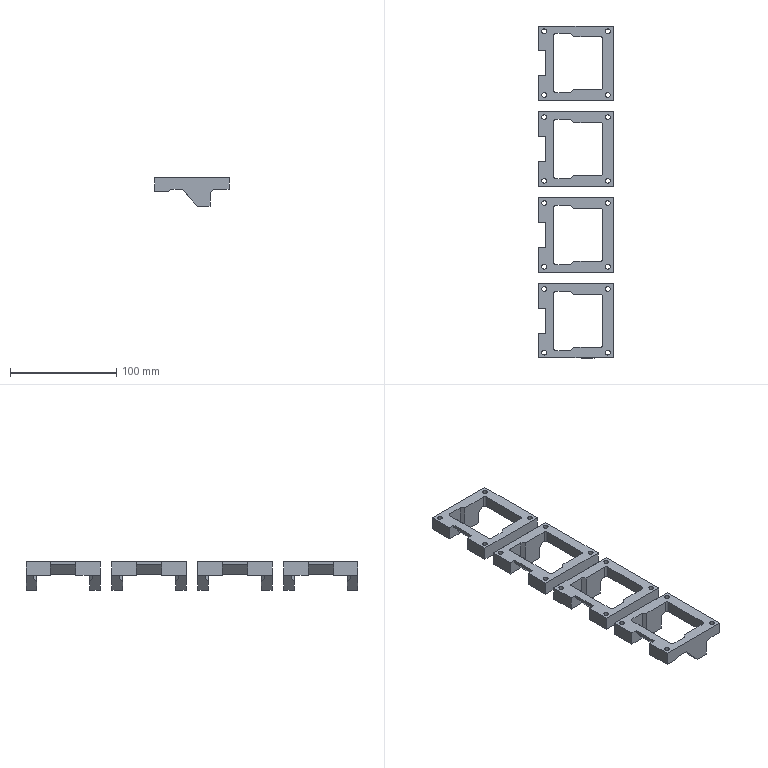NC program | NX | posted with a generic post | part box 70 x 313 x 26.9 mm
Lines 1 to 23 of 34421:
N10 G17 G21 G94 G90
(FLOOR_WALL , TOOL : D63)
N12 T01 M6
N14 G54
N16 G17 G0 G90 X206. Y-39.997 S6500 M3
N18 G43 Z30. H1
N20 Z3.
N22 G94 G1 Z0. F1500.
N24 X203.
N26 X-203.
N28 Y-17.975
N30 Y-12.599
N32 X203.
N34 Y14.8
N36 X-203.
N38 X-206.
N40 Z3.
N42 G0 Z30.
N44 M5